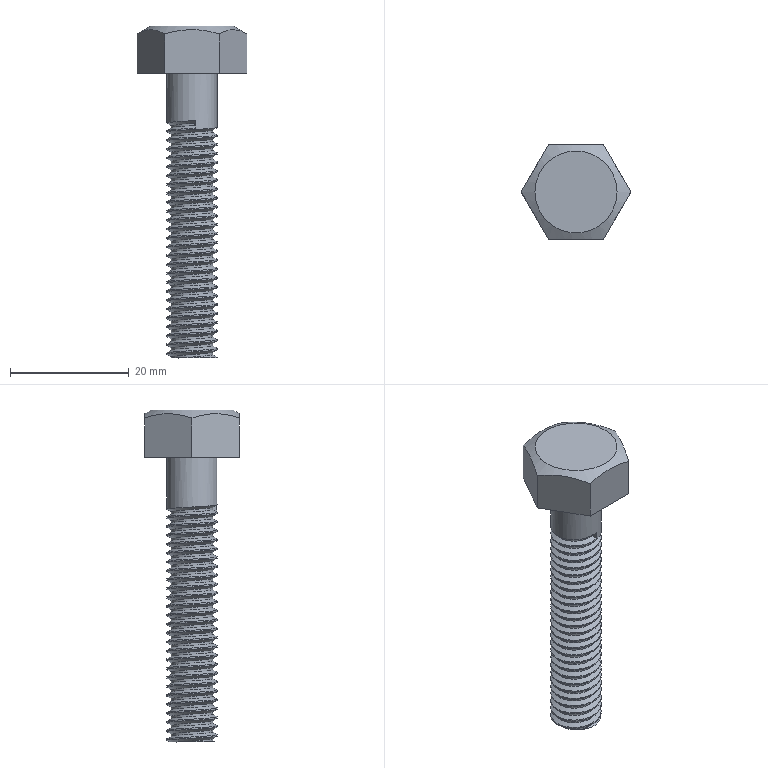Part | NX | features DATUM_CSYS 3, SKETCH 2, CYLINDER 1, EXTRUDE 1, SWP104 1, THREADS 1 | 1 solid | 41 faces | box 18.475 x 16 x 56 mm | volume 4007 mm3 | cylinder 28 | plane 10 | spline 2 | cone 1 | commonest cylinder face diameters 8.5 x27 7 x1